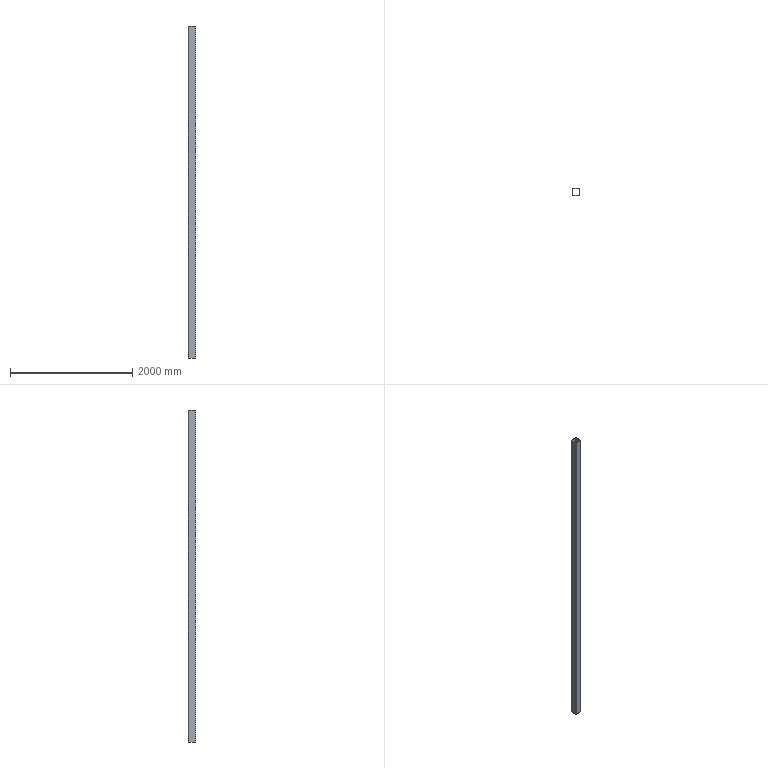Part | SolidWorks | features ICE 1, LibraryFeature 1 | 1 solid | 18 faces | box 120 x 120 x 5430 mm | volume 9854345 mm3 | plane 10 | cylinder 8 | commonest cylinder face diameters 8 x4 16 x4
STEP:
#1=CARTESIAN_POINT('',(52.,60.,-2715.));
#2=VERTEX_POINT('',#1);
#3=CARTESIAN_POINT('',(-52.,60.,-2715.));
#4=VERTEX_POINT('',#3);
#5=CARTESIAN_POINT('',(0.,60.,-2715.));
#6=DIRECTION('',(-1.,0.,0.));
#7=VECTOR('',#6,1000.);
#8=LINE('',#5,#7);
#9=EDGE_CURVE('',#2,#4,#8,.T.);
#10=ORIENTED_EDGE('',*,*,#9,.T.);
#11=CARTESIAN_POINT('',(-52.,60.,2715.));
#12=VERTEX_POINT('',#11);
#13=CARTESIAN_POINT('',(-52.,60.,2715.));
#14=DIRECTION('',(0.,0.,-1.));
#15=VECTOR('',#14,1000.);
#16=LINE('',#13,#15);
#17=EDGE_CURVE('',#12,#4,#16,.T.);
#18=ORIENTED_EDGE('',*,*,#17,.F.);
#19=CARTESIAN_POINT('',(52.,60.,2715.));
#20=VERTEX_POINT('',#19);
#21=CARTESIAN_POINT('',(0.,60.,2715.));
#22=DIRECTION('',(-1.,0.,0.));
#23=VECTOR('',#22,1000.);
#24=LINE('',#21,#23);
#25=EDGE_CURVE('',#20,#12,#24,.T.);
#26=ORIENTED_EDGE('',*,*,#25,.F.);
#27=CARTESIAN_POINT('',(52.,60.,2715.));
#28=DIRECTION('',(0.,0.,-1.));
#29=VECTOR('',#28,1000.);
#30=LINE('',#27,#29);
#31=EDGE_CURVE('',#20,#2,#30,.T.);
#32=ORIENTED_EDGE('',*,*,#31,.T.);
#33=EDGE_LOOP('',(#10,#18,#26,#32));
#34=FACE_OUTER_BOUND('',#33,.T.);
#35=CARTESIAN_POINT('',(0.,60.,2715.));
#36=DIRECTION('',(0.,-1.,0.));
#37=DIRECTION('',(0.,0.,-1.));
#38=AXIS2_PLACEMENT_3D('',#35,#36,#37);
#39=PLANE('',#38);
#40=ADVANCED_FACE('',(#34),#39,.F.);
#41=CARTESIAN_POINT('',(-60.,52.,-2715.));
#42=VERTEX_POINT('',#41);
#43=CARTESIAN_POINT('',(-52.,52.,-2715.));
#44=DIRECTION('',(0.,0.,1.));
#45=DIRECTION('',(1.,0.,0.));
#46=AXIS2_PLACEMENT_3D('',#43,#44,#45);
#47=CIRCLE('',#46,8.);
#48=EDGE_CURVE('',#4,#42,#47,.T.);
#49=ORIENTED_EDGE('',*,*,#48,.T.);
#50=CARTESIAN_POINT('',(-60.,52.,2715.));
#51=VERTEX_POINT('',#50);
#52=CARTESIAN_POINT('',(-60.,52.,2715.));
#53=DIRECTION('',(0.,0.,-1.));
#54=VECTOR('',#53,1000.);
#55=LINE('',#52,#54);
#56=EDGE_CURVE('',#51,#42,#55,.T.);
#57=ORIENTED_EDGE('',*,*,#56,.F.);
#58=CARTESIAN_POINT('',(-52.,52.,2715.));
#59=DIRECTION('',(0.,0.,1.));
#60=DIRECTION('',(1.,0.,0.));
#61=AXIS2_PLACEMENT_3D('',#58,#59,#60);
#62=CIRCLE('',#61,8.);
#63=EDGE_CURVE('',#12,#51,#62,.T.);
#64=ORIENTED_EDGE('',*,*,#63,.F.);
#65=ORIENTED_EDGE('',*,*,#17,.T.);
#66=EDGE_LOOP('',(#49,#57,#64,#65));
#67=FACE_OUTER_BOUND('',#66,.T.);
#68=CARTESIAN_POINT('',(-52.,52.,2715.));
#69=DIRECTION('',(0.,0.,-1.));
#70=DIRECTION('',(-1.,0.,0.));
#71=AXIS2_PLACEMENT_3D('',#68,#69,#70);
#72=CYLINDRICAL_SURFACE('',#71,8.);
#73=ADVANCED_FACE('',(#67),#72,.T.);
#74=CARTESIAN_POINT('',(-60.,-52.,-2715.));
#75=VERTEX_POINT('',#74);
#76=CARTESIAN_POINT('',(-60.,0.,-2715.));
#77=DIRECTION('',(0.,1.,0.));
#78=VECTOR('',#77,1000.);
#79=LINE('',#76,#78);
#80=EDGE_CURVE('',#75,#42,#79,.T.);
#81=ORIENTED_EDGE('',*,*,#80,.F.);
#82=CARTESIAN_POINT('',(-60.,-52.,2715.));
#83=VERTEX_POINT('',#82);
#84=CARTESIAN_POINT('',(-60.,-52.,2715.));
#85=DIRECTION('',(0.,0.,-1.));
#86=VECTOR('',#85,1000.);
#87=LINE('',#84,#86);
#88=EDGE_CURVE('',#83,#75,#87,.T.);
#89=ORIENTED_EDGE('',*,*,#88,.F.);
#90=CARTESIAN_POINT('',(-60.,0.,2715.));
#91=DIRECTION('',(0.,1.,0.));
#92=VECTOR('',#91,1000.);
#93=LINE('',#90,#92);
#94=EDGE_CURVE('',#83,#51,#93,.T.);
#95=ORIENTED_EDGE('',*,*,#94,.T.);
#96=ORIENTED_EDGE('',*,*,#56,.T.);
#97=EDGE_LOOP('',(#81,#89,#95,#96));
#98=FACE_OUTER_BOUND('',#97,.T.);
#99=CARTESIAN_POINT('',(-60.,0.,2715.));
#100=DIRECTION('',(-1.,0.,0.));
#101=DIRECTION('',(0.,0.,1.));
#102=AXIS2_PLACEMENT_3D('',#99,#100,#101);
#103=PLANE('',#102);
#104=ADVANCED_FACE('',(#98),#103,.T.);
#105=CARTESIAN_POINT('',(-52.,-60.,-2715.));
#106=VERTEX_POINT('',#105);
#107=CARTESIAN_POINT('',(-52.,-52.,-2715.));
#108=DIRECTION('',(0.,0.,1.));
#109=DIRECTION('',(1.,0.,0.));
#110=AXIS2_PLACEMENT_3D('',#107,#108,#109);
#111=CIRCLE('',#110,8.);
#112=EDGE_CURVE('',#75,#106,#111,.T.);
#113=ORIENTED_EDGE('',*,*,#112,.T.);
#114=CARTESIAN_POINT('',(-52.,-60.,2715.));
#115=VERTEX_POINT('',#114);
#116=CARTESIAN_POINT('',(-52.,-60.,2715.));
#117=DIRECTION('',(0.,0.,-1.));
#118=VECTOR('',#117,1000.);
#119=LINE('',#116,#118);
#120=EDGE_CURVE('',#115,#106,#119,.T.);
#121=ORIENTED_EDGE('',*,*,#120,.F.);
#122=CARTESIAN_POINT('',(-52.,-52.,2715.));
#123=DIRECTION('',(0.,0.,1.));
#124=DIRECTION('',(1.,0.,0.));
#125=AXIS2_PLACEMENT_3D('',#122,#123,#124);
#126=CIRCLE('',#125,8.);
#127=EDGE_CURVE('',#83,#115,#126,.T.);
#128=ORIENTED_EDGE('',*,*,#127,.F.);
#129=ORIENTED_EDGE('',*,*,#88,.T.);
#130=EDGE_LOOP('',(#113,#121,#128,#129));
#131=FACE_OUTER_BOUND('',#130,.T.);
#132=CARTESIAN_POINT('',(-52.,-52.,2715.));
#133=DIRECTION('',(0.,0.,-1.));
#134=DIRECTION('',(-1.,0.,0.));
#135=AXIS2_PLACEMENT_3D('',#132,#133,#134);
#136=CYLINDRICAL_SURFACE('',#135,8.);
#137=ADVANCED_FACE('',(#131),#136,.T.);
#138=CARTESIAN_POINT('',(52.,-60.,-2715.));
#139=VERTEX_POINT('',#138);
#140=CARTESIAN_POINT('',(0.,-60.,-2715.));
#141=DIRECTION('',(1.,0.,0.));
#142=VECTOR('',#141,1000.);
#143=LINE('',#140,#142);
#144=EDGE_CURVE('',#106,#139,#143,.T.);
#145=ORIENTED_EDGE('',*,*,#144,.T.);
#146=CARTESIAN_POINT('',(52.,-60.,2715.));
#147=VERTEX_POINT('',#146);
#148=CARTESIAN_POINT('',(52.,-60.,2715.));
#149=DIRECTION('',(0.,0.,-1.));
#150=VECTOR('',#149,1000.);
#151=LINE('',#148,#150);
#152=EDGE_CURVE('',#147,#139,#151,.T.);
#153=ORIENTED_EDGE('',*,*,#152,.F.);
#154=CARTESIAN_POINT('',(0.,-60.,2715.));
#155=DIRECTION('',(1.,0.,0.));
#156=VECTOR('',#155,1000.);
#157=LINE('',#154,#156);
#158=EDGE_CURVE('',#115,#147,#157,.T.);
#159=ORIENTED_EDGE('',*,*,#158,.F.);
#160=ORIENTED_EDGE('',*,*,#120,.T.);
#161=EDGE_LOOP('',(#145,#153,#159,#160));
#162=FACE_OUTER_BOUND('',#161,.T.);
#163=CARTESIAN_POINT('',(0.,-60.,2715.));
#164=DIRECTION('',(0.,1.,0.));
#165=DIRECTION('',(0.,0.,1.));
#166=AXIS2_PLACEMENT_3D('',#163,#164,#165);
#167=PLANE('',#166);
#168=ADVANCED_FACE('',(#162),#167,.F.);
#169=CARTESIAN_POINT('',(60.,-52.,-2715.));
#170=VERTEX_POINT('',#169);
#171=CARTESIAN_POINT('',(52.,-52.,-2715.));
#172=DIRECTION('',(0.,0.,1.));
#173=DIRECTION('',(1.,0.,0.));
#174=AXIS2_PLACEMENT_3D('',#171,#172,#173);
#175=CIRCLE('',#174,8.);
#176=EDGE_CURVE('',#139,#170,#175,.T.);
#177=ORIENTED_EDGE('',*,*,#176,.T.);
#178=CARTESIAN_POINT('',(60.,-52.,2715.));
#179=VERTEX_POINT('',#178);
#180=CARTESIAN_POINT('',(60.,-52.,2715.));
#181=DIRECTION('',(0.,0.,-1.));
#182=VECTOR('',#181,1000.);
#183=LINE('',#180,#182);
#184=EDGE_CURVE('',#179,#170,#183,.T.);
#185=ORIENTED_EDGE('',*,*,#184,.F.);
#186=CARTESIAN_POINT('',(52.,-52.,2715.));
#187=DIRECTION('',(0.,0.,1.));
#188=DIRECTION('',(1.,0.,0.));
#189=AXIS2_PLACEMENT_3D('',#186,#187,#188);
#190=CIRCLE('',#189,8.);
#191=EDGE_CURVE('',#147,#179,#190,.T.);
#192=ORIENTED_EDGE('',*,*,#191,.F.);
#193=ORIENTED_EDGE('',*,*,#152,.T.);
#194=EDGE_LOOP('',(#177,#185,#192,#193));
#195=FACE_OUTER_BOUND('',#194,.T.);
#196=CARTESIAN_POINT('',(52.,-52.,2715.));
#197=DIRECTION('',(0.,0.,-1.));
#198=DIRECTION('',(-1.,0.,0.));
#199=AXIS2_PLACEMENT_3D('',#196,#197,#198);
#200=CYLINDRICAL_SURFACE('',#199,8.);
#201=ADVANCED_FACE('',(#195),#200,.T.);
#202=CARTESIAN_POINT('',(60.,52.,-2715.));
#203=VERTEX_POINT('',#202);
#204=CARTESIAN_POINT('',(60.,0.,-2715.));
#205=DIRECTION('',(0.,-1.,0.));
#206=VECTOR('',#205,1000.);
#207=LINE('',#204,#206);
#208=EDGE_CURVE('',#203,#170,#207,.T.);
#209=ORIENTED_EDGE('',*,*,#208,.F.);
#210=CARTESIAN_POINT('',(60.,52.,2715.));
#211=VERTEX_POINT('',#210);
#212=CARTESIAN_POINT('',(60.,52.,2715.));
#213=DIRECTION('',(0.,0.,-1.));
#214=VECTOR('',#213,1000.);
#215=LINE('',#212,#214);
#216=EDGE_CURVE('',#211,#203,#215,.T.);
#217=ORIENTED_EDGE('',*,*,#216,.F.);
#218=CARTESIAN_POINT('',(60.,0.,2715.));
#219=DIRECTION('',(0.,-1.,0.));
#220=VECTOR('',#219,1000.);
#221=LINE('',#218,#220);
#222=EDGE_CURVE('',#211,#179,#221,.T.);
#223=ORIENTED_EDGE('',*,*,#222,.T.);
#224=ORIENTED_EDGE('',*,*,#184,.T.);
#225=EDGE_LOOP('',(#209,#217,#223,#224));
#226=FACE_OUTER_BOUND('',#225,.T.);
#227=CARTESIAN_POINT('',(60.,0.,2715.));
#228=DIRECTION('',(1.,0.,0.));
#229=DIRECTION('',(0.,0.,-1.));
#230=AXIS2_PLACEMENT_3D('',#227,#228,#229);
#231=PLANE('',#230);
#232=ADVANCED_FACE('',(#226),#231,.T.);
#233=CARTESIAN_POINT('',(-56.,-52.,-2715.));
#234=VERTEX_POINT('',#233);
#235=CARTESIAN_POINT('',(-52.,-56.,-2715.));
#236=VERTEX_POINT('',#235);
#237=CARTESIAN_POINT('',(-52.,-52.,-2715.));
#238=DIRECTION('',(0.,0.,1.));
#239=DIRECTION('',(1.,0.,0.));
#240=AXIS2_PLACEMENT_3D('',#237,#238,#239);
#241=CIRCLE('',#240,4.);
#242=EDGE_CURVE('',#234,#236,#241,.T.);
#243=ORIENTED_EDGE('',*,*,#242,.F.);
#244=CARTESIAN_POINT('',(-56.,-52.,2715.));
#245=VERTEX_POINT('',#244);
#246=CARTESIAN_POINT('',(-56.,-52.,2715.));
#247=DIRECTION('',(0.,0.,-1.));
#248=VECTOR('',#247,1000.);
#249=LINE('',#246,#248);
#250=EDGE_CURVE('',#245,#234,#249,.T.);
#251=ORIENTED_EDGE('',*,*,#250,.F.);
#252=CARTESIAN_POINT('',(-52.,-56.,2715.));
#253=VERTEX_POINT('',#252);
#254=CARTESIAN_POINT('',(-52.,-52.,2715.));
#255=DIRECTION('',(0.,0.,1.));
#256=DIRECTION('',(1.,0.,0.));
#257=AXIS2_PLACEMENT_3D('',#254,#255,#256);
#258=CIRCLE('',#257,4.);
#259=EDGE_CURVE('',#245,#253,#258,.T.);
#260=ORIENTED_EDGE('',*,*,#259,.T.);
#261=CARTESIAN_POINT('',(-52.,-56.,2715.));
#262=DIRECTION('',(0.,0.,-1.));
#263=VECTOR('',#262,1000.);
#264=LINE('',#261,#263);
#265=EDGE_CURVE('',#253,#236,#264,.T.);
#266=ORIENTED_EDGE('',*,*,#265,.T.);
#267=EDGE_LOOP('',(#243,#251,#260,#266));
#268=FACE_OUTER_BOUND('',#267,.T.);
#269=CARTESIAN_POINT('',(-52.,-52.,2715.));
#270=DIRECTION('',(0.,0.,-1.));
#271=DIRECTION('',(-1.,0.,0.));
#272=AXIS2_PLACEMENT_3D('',#269,#270,#271);
#273=CYLINDRICAL_SURFACE('',#272,4.);
#274=ADVANCED_FACE('',(#268),#273,.F.);
#275=CARTESIAN_POINT('',(-56.,52.,-2715.));
#276=VERTEX_POINT('',#275);
#277=CARTESIAN_POINT('',(-56.,0.,-2715.));
#278=DIRECTION('',(0.,1.,0.));
#279=VECTOR('',#278,1000.);
#280=LINE('',#277,#279);
#281=EDGE_CURVE('',#234,#276,#280,.T.);
#282=ORIENTED_EDGE('',*,*,#281,.T.);
#283=CARTESIAN_POINT('',(-56.,52.,2715.));
#284=VERTEX_POINT('',#283);
#285=CARTESIAN_POINT('',(-56.,52.,2715.));
#286=DIRECTION('',(0.,0.,-1.));
#287=VECTOR('',#286,1000.);
#288=LINE('',#285,#287);
#289=EDGE_CURVE('',#284,#276,#288,.T.);
#290=ORIENTED_EDGE('',*,*,#289,.F.);
#291=CARTESIAN_POINT('',(-56.,0.,2715.));
#292=DIRECTION('',(0.,1.,0.));
#293=VECTOR('',#292,1000.);
#294=LINE('',#291,#293);
#295=EDGE_CURVE('',#245,#284,#294,.T.);
#296=ORIENTED_EDGE('',*,*,#295,.F.);
#297=ORIENTED_EDGE('',*,*,#250,.T.);
#298=EDGE_LOOP('',(#282,#290,#296,#297));
#299=FACE_OUTER_BOUND('',#298,.T.);
#300=CARTESIAN_POINT('',(-56.,0.,2715.));
#301=DIRECTION('',(-1.,0.,0.));
#302=DIRECTION('',(0.,0.,1.));
#303=AXIS2_PLACEMENT_3D('',#300,#301,#302);
#304=PLANE('',#303);
#305=ADVANCED_FACE('',(#299),#304,.F.);
#306=CARTESIAN_POINT('',(-52.,56.,-2715.));
#307=VERTEX_POINT('',#306);
#308=CARTESIAN_POINT('',(-52.,52.,-2715.));
#309=DIRECTION('',(0.,0.,1.));
#310=DIRECTION('',(1.,0.,0.));
#311=AXIS2_PLACEMENT_3D('',#308,#309,#310);
#312=CIRCLE('',#311,4.);
#313=EDGE_CURVE('',#307,#276,#312,.T.);
#314=ORIENTED_EDGE('',*,*,#313,.F.);
#315=CARTESIAN_POINT('',(-52.,56.,2715.));
#316=VERTEX_POINT('',#315);
#317=CARTESIAN_POINT('',(-52.,56.,2715.));
#318=DIRECTION('',(0.,0.,-1.));
#319=VECTOR('',#318,1000.);
#320=LINE('',#317,#319);
#321=EDGE_CURVE('',#316,#307,#320,.T.);
#322=ORIENTED_EDGE('',*,*,#321,.F.);
#323=CARTESIAN_POINT('',(-52.,52.,2715.));
#324=DIRECTION('',(0.,0.,1.));
#325=DIRECTION('',(1.,0.,0.));
#326=AXIS2_PLACEMENT_3D('',#323,#324,#325);
#327=CIRCLE('',#326,4.);
#328=EDGE_CURVE('',#316,#284,#327,.T.);
#329=ORIENTED_EDGE('',*,*,#328,.T.);
#330=ORIENTED_EDGE('',*,*,#289,.T.);
#331=EDGE_LOOP('',(#314,#322,#329,#330));
#332=FACE_OUTER_BOUND('',#331,.T.);
#333=CARTESIAN_POINT('',(-52.,52.,2715.));
#334=DIRECTION('',(0.,0.,-1.));
#335=DIRECTION('',(-1.,0.,0.));
#336=AXIS2_PLACEMENT_3D('',#333,#334,#335);
#337=CYLINDRICAL_SURFACE('',#336,4.);
#338=ADVANCED_FACE('',(#332),#337,.F.);
#339=CARTESIAN_POINT('',(52.,56.,-2715.));
#340=VERTEX_POINT('',#339);
#341=CARTESIAN_POINT('',(0.,56.,-2715.));
#342=DIRECTION('',(-1.,0.,0.));
#343=VECTOR('',#342,1000.);
#344=LINE('',#341,#343);
#345=EDGE_CURVE('',#340,#307,#344,.T.);
#346=ORIENTED_EDGE('',*,*,#345,.F.);
#347=CARTESIAN_POINT('',(52.,56.,2715.));
#348=VERTEX_POINT('',#347);
#349=CARTESIAN_POINT('',(52.,56.,2715.));
#350=DIRECTION('',(0.,0.,-1.));
#351=VECTOR('',#350,1000.);
#352=LINE('',#349,#351);
#353=EDGE_CURVE('',#348,#340,#352,.T.);
#354=ORIENTED_EDGE('',*,*,#353,.F.);
#355=CARTESIAN_POINT('',(0.,56.,2715.));
#356=DIRECTION('',(-1.,0.,0.));
#357=VECTOR('',#356,1000.);
#358=LINE('',#355,#357);
#359=EDGE_CURVE('',#348,#316,#358,.T.);
#360=ORIENTED_EDGE('',*,*,#359,.T.);
#361=ORIENTED_EDGE('',*,*,#321,.T.);
#362=EDGE_LOOP('',(#346,#354,#360,#361));
#363=FACE_OUTER_BOUND('',#362,.T.);
#364=CARTESIAN_POINT('',(0.,56.,2715.));
#365=DIRECTION('',(0.,-1.,0.));
#366=DIRECTION('',(0.,0.,-1.));
#367=AXIS2_PLACEMENT_3D('',#364,#365,#366);
#368=PLANE('',#367);
#369=ADVANCED_FACE('',(#363),#368,.T.);
#370=CARTESIAN_POINT('',(56.,52.,-2715.));
#371=VERTEX_POINT('',#370);
#372=CARTESIAN_POINT('',(52.,52.,-2715.));
#373=DIRECTION('',(0.,0.,1.));
#374=DIRECTION('',(1.,0.,0.));
#375=AXIS2_PLACEMENT_3D('',#372,#373,#374);
#376=CIRCLE('',#375,4.);
#377=EDGE_CURVE('',#371,#340,#376,.T.);
#378=ORIENTED_EDGE('',*,*,#377,.F.);
#379=CARTESIAN_POINT('',(56.,52.,2715.));
#380=VERTEX_POINT('',#379);
#381=CARTESIAN_POINT('',(56.,52.,2715.));
#382=DIRECTION('',(0.,0.,-1.));
#383=VECTOR('',#382,1000.);
#384=LINE('',#381,#383);
#385=EDGE_CURVE('',#380,#371,#384,.T.);
#386=ORIENTED_EDGE('',*,*,#385,.F.);
#387=CARTESIAN_POINT('',(52.,52.,2715.));
#388=DIRECTION('',(0.,0.,1.));
#389=DIRECTION('',(1.,0.,0.));
#390=AXIS2_PLACEMENT_3D('',#387,#388,#389);
#391=CIRCLE('',#390,4.);
#392=EDGE_CURVE('',#380,#348,#391,.T.);
#393=ORIENTED_EDGE('',*,*,#392,.T.);
#394=ORIENTED_EDGE('',*,*,#353,.T.);
#395=EDGE_LOOP('',(#378,#386,#393,#394));
#396=FACE_OUTER_BOUND('',#395,.T.);
#397=CARTESIAN_POINT('',(52.,52.,2715.));
#398=DIRECTION('',(0.,0.,-1.));
#399=DIRECTION('',(-1.,0.,0.));
#400=AXIS2_PLACEMENT_3D('',#397,#398,#399);
#401=CYLINDRICAL_SURFACE('',#400,4.);
#402=ADVANCED_FACE('',(#396),#401,.F.);
#403=CARTESIAN_POINT('',(56.,-52.,-2715.));
#404=VERTEX_POINT('',#403);
#405=CARTESIAN_POINT('',(56.,0.,-2715.));
#406=DIRECTION('',(0.,-1.,0.));
#407=VECTOR('',#406,1000.);
#408=LINE('',#405,#407);
#409=EDGE_CURVE('',#371,#404,#408,.T.);
#410=ORIENTED_EDGE('',*,*,#409,.T.);
#411=CARTESIAN_POINT('',(56.,-52.,2715.));
#412=VERTEX_POINT('',#411);
#413=CARTESIAN_POINT('',(56.,-52.,2715.));
#414=DIRECTION('',(0.,0.,-1.));
#415=VECTOR('',#414,1000.);
#416=LINE('',#413,#415);
#417=EDGE_CURVE('',#412,#404,#416,.T.);
#418=ORIENTED_EDGE('',*,*,#417,.F.);
#419=CARTESIAN_POINT('',(56.,0.,2715.));
#420=DIRECTION('',(0.,-1.,0.));
#421=VECTOR('',#420,1000.);
#422=LINE('',#419,#421);
#423=EDGE_CURVE('',#380,#412,#422,.T.);
#424=ORIENTED_EDGE('',*,*,#423,.F.);
#425=ORIENTED_EDGE('',*,*,#385,.T.);
#426=EDGE_LOOP('',(#410,#418,#424,#425));
#427=FACE_OUTER_BOUND('',#426,.T.);
#428=CARTESIAN_POINT('',(56.,0.,2715.));
#429=DIRECTION('',(1.,0.,0.));
#430=DIRECTION('',(0.,0.,-1.));
#431=AXIS2_PLACEMENT_3D('',#428,#429,#430);
#432=PLANE('',#431);
#433=ADVANCED_FACE('',(#427),#432,.F.);
#434=CARTESIAN_POINT('',(52.,-56.,-2715.));
#435=VERTEX_POINT('',#434);
#436=CARTESIAN_POINT('',(52.,-52.,-2715.));
#437=DIRECTION('',(0.,0.,1.));
#438=DIRECTION('',(1.,0.,0.));
#439=AXIS2_PLACEMENT_3D('',#436,#437,#438);
#440=CIRCLE('',#439,4.);
#441=EDGE_CURVE('',#435,#404,#440,.T.);
#442=ORIENTED_EDGE('',*,*,#441,.F.);
#443=CARTESIAN_POINT('',(52.,-56.,2715.));
#444=VERTEX_POINT('',#443);
#445=CARTESIAN_POINT('',(52.,-56.,2715.));
#446=DIRECTION('',(0.,0.,-1.));
#447=VECTOR('',#446,1000.);
#448=LINE('',#445,#447);
#449=EDGE_CURVE('',#444,#435,#448,.T.);
#450=ORIENTED_EDGE('',*,*,#449,.F.);
#451=CARTESIAN_POINT('',(52.,-52.,2715.));
#452=DIRECTION('',(0.,0.,1.));
#453=DIRECTION('',(1.,0.,0.));
#454=AXIS2_PLACEMENT_3D('',#451,#452,#453);
#455=CIRCLE('',#454,4.);
#456=EDGE_CURVE('',#444,#412,#455,.T.);
#457=ORIENTED_EDGE('',*,*,#456,.T.);
#458=ORIENTED_EDGE('',*,*,#417,.T.);
#459=EDGE_LOOP('',(#442,#450,#457,#458));
#460=FACE_OUTER_BOUND('',#459,.T.);
#461=CARTESIAN_POINT('',(52.,-52.,2715.));
#462=DIRECTION('',(0.,0.,-1.));
#463=DIRECTION('',(-1.,0.,0.));
#464=AXIS2_PLACEMENT_3D('',#461,#462,#463);
#465=CYLINDRICAL_SURFACE('',#464,4.);
#466=ADVANCED_FACE('',(#460),#465,.F.);
#467=CARTESIAN_POINT('',(0.,-56.,-2715.));
#468=DIRECTION('',(1.,0.,0.));
#469=VECTOR('',#468,1000.);
#470=LINE('',#467,#469);
#471=EDGE_CURVE('',#236,#435,#470,.T.);
#472=ORIENTED_EDGE('',*,*,#471,.F.);
#473=ORIENTED_EDGE('',*,*,#265,.F.);
#474=CARTESIAN_POINT('',(0.,-56.,2715.));
#475=DIRECTION('',(1.,0.,0.));
#476=VECTOR('',#475,1000.);
#477=LINE('',#474,#476);
#478=EDGE_CURVE('',#253,#444,#477,.T.);
#479=ORIENTED_EDGE('',*,*,#478,.T.);
#480=ORIENTED_EDGE('',*,*,#449,.T.);
#481=EDGE_LOOP('',(#472,#473,#479,#480));
#482=FACE_OUTER_BOUND('',#481,.T.);
#483=CARTESIAN_POINT('',(0.,-56.,2715.));
#484=DIRECTION('',(0.,1.,0.));
#485=DIRECTION('',(0.,0.,1.));
#486=AXIS2_PLACEMENT_3D('',#483,#484,#485);
#487=PLANE('',#486);
#488=ADVANCED_FACE('',(#482),#487,.T.);
#489=CARTESIAN_POINT('',(52.,52.,-2715.));
#490=DIRECTION('',(0.,0.,1.));
#491=DIRECTION('',(1.,0.,0.));
#492=AXIS2_PLACEMENT_3D('',#489,#490,#491);
#493=CIRCLE('',#492,8.);
#494=EDGE_CURVE('',#203,#2,#493,.T.);
#495=ORIENTED_EDGE('',*,*,#494,.T.);
#496=ORIENTED_EDGE('',*,*,#31,.F.);
#497=CARTESIAN_POINT('',(52.,52.,2715.));
#498=DIRECTION('',(0.,0.,1.));
#499=DIRECTION('',(1.,0.,0.));
#500=AXIS2_PLACEMENT_3D('',#497,#498,#499);
#501=CIRCLE('',#500,8.);
#502=EDGE_CURVE('',#211,#20,#501,.T.);
#503=ORIENTED_EDGE('',*,*,#502,.F.);
#504=ORIENTED_EDGE('',*,*,#216,.T.);
#505=EDGE_LOOP('',(#495,#496,#503,#504));
#506=FACE_OUTER_BOUND('',#505,.T.);
#507=CARTESIAN_POINT('',(52.,52.,2715.));
#508=DIRECTION('',(0.,0.,-1.));
#509=DIRECTION('',(-1.,0.,0.));
#510=AXIS2_PLACEMENT_3D('',#507,#508,#509);
#511=CYLINDRICAL_SURFACE('',#510,8.);
#512=ADVANCED_FACE('',(#506),#511,.T.);
#513=ORIENTED_EDGE('',*,*,#259,.F.);
#514=ORIENTED_EDGE('',*,*,#295,.T.);
#515=ORIENTED_EDGE('',*,*,#328,.F.);
#516=ORIENTED_EDGE('',*,*,#359,.F.);
#517=ORIENTED_EDGE('',*,*,#392,.F.);
#518=ORIENTED_EDGE('',*,*,#423,.T.);
#519=ORIENTED_EDGE('',*,*,#456,.F.);
#520=ORIENTED_EDGE('',*,*,#478,.F.);
#521=EDGE_LOOP('',(#513,#514,#515,#516,#517,#518,#519,#520));
#522=FACE_BOUND('',#521,.T.);
#523=ORIENTED_EDGE('',*,*,#25,.T.);
#524=ORIENTED_EDGE('',*,*,#63,.T.);
#525=ORIENTED_EDGE('',*,*,#94,.F.);
#526=ORIENTED_EDGE('',*,*,#127,.T.);
#527=ORIENTED_EDGE('',*,*,#158,.T.);
#528=ORIENTED_EDGE('',*,*,#191,.T.);
#529=ORIENTED_EDGE('',*,*,#222,.F.);
#530=ORIENTED_EDGE('',*,*,#502,.T.);
#531=EDGE_LOOP('',(#523,#524,#525,#526,#527,#528,#529,#530));
#532=FACE_OUTER_BOUND('',#531,.T.);
#533=CARTESIAN_POINT('',(0.,0.,2715.));
#534=DIRECTION('',(0.,0.,1.));
#535=DIRECTION('',(1.,0.,0.));
#536=AXIS2_PLACEMENT_3D('',#533,#534,#535);
#537=PLANE('',#536);
#538=ADVANCED_FACE('',(#522,#532),#537,.T.);
#539=ORIENTED_EDGE('',*,*,#242,.T.);
#540=ORIENTED_EDGE('',*,*,#471,.T.);
#541=ORIENTED_EDGE('',*,*,#441,.T.);
#542=ORIENTED_EDGE('',*,*,#409,.F.);
#543=ORIENTED_EDGE('',*,*,#377,.T.);
#544=ORIENTED_EDGE('',*,*,#345,.T.);
#545=ORIENTED_EDGE('',*,*,#313,.T.);
#546=ORIENTED_EDGE('',*,*,#281,.F.);
#547=EDGE_LOOP('',(#539,#540,#541,#542,#543,#544,#545,#546));
#548=FACE_BOUND('',#547,.T.);
#549=ORIENTED_EDGE('',*,*,#9,.F.);
#550=ORIENTED_EDGE('',*,*,#494,.F.);
#551=ORIENTED_EDGE('',*,*,#208,.T.);
#552=ORIENTED_EDGE('',*,*,#176,.F.);
#553=ORIENTED_EDGE('',*,*,#144,.F.);
#554=ORIENTED_EDGE('',*,*,#112,.F.);
#555=ORIENTED_EDGE('',*,*,#80,.T.);
#556=ORIENTED_EDGE('',*,*,#48,.F.);
#557=EDGE_LOOP('',(#549,#550,#551,#552,#553,#554,#555,#556));
#558=FACE_OUTER_BOUND('',#557,.T.);
#559=CARTESIAN_POINT('',(0.,0.,-2715.));
#560=DIRECTION('',(0.,0.,1.));
#561=DIRECTION('',(1.,0.,0.));
#562=AXIS2_PLACEMENT_3D('',#559,#560,#561);
#563=PLANE('',#562);
#564=ADVANCED_FACE('',(#548,#558),#563,.F.);
#565=CLOSED_SHELL('',(#40,#73,#104,#137,#168,#201,#232,#274,#305,#338,#369,#402,#433,#466,#488,#512,#538,#564));
#566=MANIFOLD_SOLID_BREP('',#565);
#567=CARTESIAN_POINT('',(0.,0.,0.));
#568=DIRECTION('',(0.,0.,1.));
#569=DIRECTION('',(1.,0.,0.));
#570=AXIS2_PLACEMENT_3D('',#567,#568,#569);
#571=(LENGTH_UNIT()NAMED_UNIT(*)SI_UNIT(.MILLI.,.METRE.));
#572=UNCERTAINTY_MEASURE_WITH_UNIT(LENGTH_MEASURE(0.00001),#571,'','');
#573=(NAMED_UNIT(*)PLANE_ANGLE_UNIT()SI_UNIT($,.RADIAN.));
#574=(NAMED_UNIT(*)SI_UNIT($,.STERADIAN.)SOLID_ANGLE_UNIT());
#575=(GEOMETRIC_REPRESENTATION_CONTEXT(3)GLOBAL_UNCERTAINTY_ASSIGNED_CONTEXT((#572))GLOBAL_UNIT_ASSIGNED_CONTEXT((#571,#573,#574))REPRESENTATION_CONTEXT('',''));
#576=ADVANCED_BREP_SHAPE_REPRESENTATION('',(#566,#570),#575);